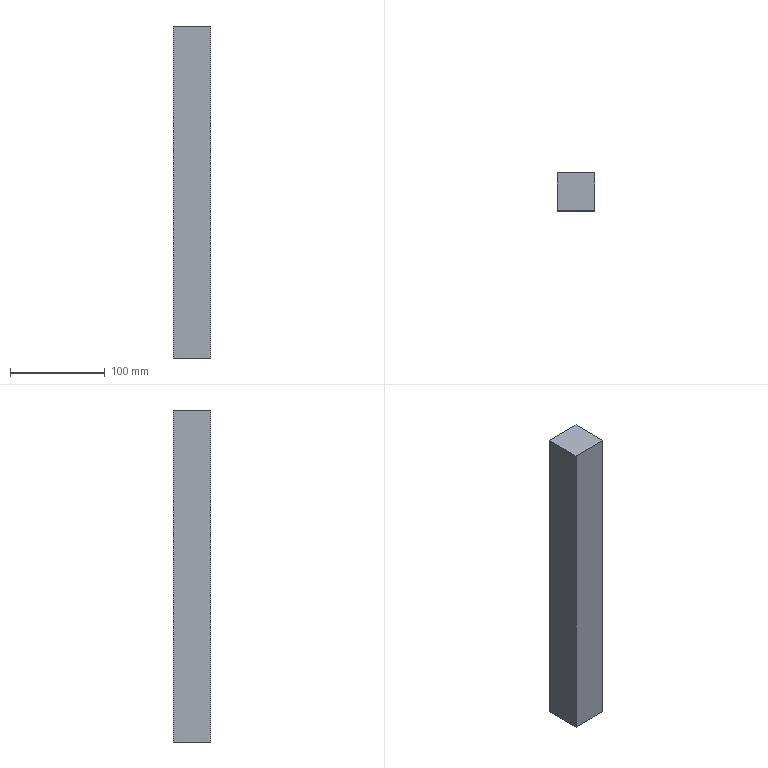Part | STEP file | Profile | 1 solid | 6 faces | box 40 x 40 x 350 mm | volume 560000 mm3 | plane 6
STEP:
#1=CARTESIAN_POINT('',(0.,0.,0.));
#2=DIRECTION('',(0.,0.,1.));
#3=DIRECTION('',(1.,0.,0.));
#4=AXIS2_PLACEMENT_3D('',#1,#2,#3);
#5=CARTESIAN_POINT('',(20.,-20.,350.));
#6=VERTEX_POINT('',#5);
#7=CARTESIAN_POINT('',(20.,-20.,0.));
#8=VERTEX_POINT('',#7);
#9=CARTESIAN_POINT('',(20.,-20.,350.));
#10=DIRECTION('',(0.,0.,-1.));
#11=VECTOR('',#10,1.);
#12=LINE('',#9,#11);
#13=CARTESIAN_POINT('',(-20.,-20.,350.));
#14=DIRECTION('',(0.,1.,0.));
#15=DIRECTION('',(0.,0.,1.));
#16=AXIS2_PLACEMENT_3D('',#13,#14,#15);
#17=PLANE('',#16);
#18=CARTESIAN_POINT('',(0.,40.));
#19=DIRECTION('',(-1.,0.));
#20=VECTOR('',#19,1.);
#21=LINE('',#18,#20);
#22=(GEOMETRIC_REPRESENTATION_CONTEXT(2)PARAMETRIC_REPRESENTATION_CONTEXT()REPRESENTATION_CONTEXT('',''));
#23=DEFINITIONAL_REPRESENTATION('',(#21),#22);
#24=PCURVE('',#17,#23);
#25=CARTESIAN_POINT('',(20.,20.,350.));
#26=DIRECTION('',(-1.,0.,0.));
#27=DIRECTION('',(0.,-1.,0.));
#28=AXIS2_PLACEMENT_3D('',#25,#26,#27);
#29=PLANE('',#28);
#30=CARTESIAN_POINT('',(40.,0.));
#31=DIRECTION('',(0.,-1.));
#32=VECTOR('',#31,1.);
#33=LINE('',#30,#32);
#34=(GEOMETRIC_REPRESENTATION_CONTEXT(2)PARAMETRIC_REPRESENTATION_CONTEXT()REPRESENTATION_CONTEXT('',''));
#35=DEFINITIONAL_REPRESENTATION('',(#33),#34);
#36=PCURVE('',#29,#35);
#37=SURFACE_CURVE('',#12,(#24,#36),.PCURVE_S1.);
#38=EDGE_CURVE('',#6,#8,#37,.T.);
#39=ORIENTED_EDGE('',*,*,#38,.F.);
#40=CARTESIAN_POINT('',(-20.,-20.,350.));
#41=VERTEX_POINT('',#40);
#42=CARTESIAN_POINT('',(-20.,-20.,350.));
#43=DIRECTION('',(1.,0.,0.));
#44=VECTOR('',#43,1.);
#45=LINE('',#42,#44);
#46=CARTESIAN_POINT('',(0.,0.));
#47=DIRECTION('',(0.,1.));
#48=VECTOR('',#47,1.);
#49=LINE('',#46,#48);
#50=(GEOMETRIC_REPRESENTATION_CONTEXT(2)PARAMETRIC_REPRESENTATION_CONTEXT()REPRESENTATION_CONTEXT('',''));
#51=DEFINITIONAL_REPRESENTATION('',(#49),#50);
#52=PCURVE('',#17,#51);
#53=CARTESIAN_POINT('',(0.,0.,350.));
#54=DIRECTION('',(0.,0.,1.));
#55=DIRECTION('',(1.,0.,0.));
#56=AXIS2_PLACEMENT_3D('',#53,#54,#55);
#57=PLANE('',#56);
#58=CARTESIAN_POINT('',(-20.,-20.));
#59=DIRECTION('',(1.,0.));
#60=VECTOR('',#59,1.);
#61=LINE('',#58,#60);
#62=(GEOMETRIC_REPRESENTATION_CONTEXT(2)PARAMETRIC_REPRESENTATION_CONTEXT()REPRESENTATION_CONTEXT('',''));
#63=DEFINITIONAL_REPRESENTATION('',(#61),#62);
#64=PCURVE('',#57,#63);
#65=SURFACE_CURVE('',#45,(#52,#64),.PCURVE_S1.);
#66=EDGE_CURVE('',#41,#6,#65,.T.);
#67=ORIENTED_EDGE('',*,*,#66,.F.);
#68=CARTESIAN_POINT('',(-20.,-20.,0.));
#69=VERTEX_POINT('',#68);
#70=CARTESIAN_POINT('',(-20.,-20.,350.));
#71=DIRECTION('',(0.,0.,1.));
#72=VECTOR('',#71,1.);
#73=LINE('',#70,#72);
#74=CARTESIAN_POINT('',(0.,0.));
#75=DIRECTION('',(1.,0.));
#76=VECTOR('',#75,1.);
#77=LINE('',#74,#76);
#78=(GEOMETRIC_REPRESENTATION_CONTEXT(2)PARAMETRIC_REPRESENTATION_CONTEXT()REPRESENTATION_CONTEXT('',''));
#79=DEFINITIONAL_REPRESENTATION('',(#77),#78);
#80=PCURVE('',#17,#79);
#81=CARTESIAN_POINT('',(-20.,20.,350.));
#82=DIRECTION('',(1.,0.,0.));
#83=DIRECTION('',(0.,1.,0.));
#84=AXIS2_PLACEMENT_3D('',#81,#82,#83);
#85=PLANE('',#84);
#86=CARTESIAN_POINT('',(-40.,0.));
#87=DIRECTION('',(0.,1.));
#88=VECTOR('',#87,1.);
#89=LINE('',#86,#88);
#90=(GEOMETRIC_REPRESENTATION_CONTEXT(2)PARAMETRIC_REPRESENTATION_CONTEXT()REPRESENTATION_CONTEXT('',''));
#91=DEFINITIONAL_REPRESENTATION('',(#89),#90);
#92=PCURVE('',#85,#91);
#93=SURFACE_CURVE('',#73,(#80,#92),.PCURVE_S1.);
#94=EDGE_CURVE('',#69,#41,#93,.T.);
#95=ORIENTED_EDGE('',*,*,#94,.F.);
#96=CARTESIAN_POINT('',(-20.,-20.,0.));
#97=DIRECTION('',(-1.,0.,0.));
#98=VECTOR('',#97,1.);
#99=LINE('',#96,#98);
#100=CARTESIAN_POINT('',(-350.,0.));
#101=DIRECTION('',(0.,-1.));
#102=VECTOR('',#101,1.);
#103=LINE('',#100,#102);
#104=(GEOMETRIC_REPRESENTATION_CONTEXT(2)PARAMETRIC_REPRESENTATION_CONTEXT()REPRESENTATION_CONTEXT('',''));
#105=DEFINITIONAL_REPRESENTATION('',(#103),#104);
#106=PCURVE('',#17,#105);
#107=CARTESIAN_POINT('',(0.,0.,0.));
#108=DIRECTION('',(0.,0.,1.));
#109=DIRECTION('',(1.,0.,0.));
#110=AXIS2_PLACEMENT_3D('',#107,#108,#109);
#111=PLANE('',#110);
#112=CARTESIAN_POINT('',(-20.,-20.));
#113=DIRECTION('',(-1.,0.));
#114=VECTOR('',#113,1.);
#115=LINE('',#112,#114);
#116=(GEOMETRIC_REPRESENTATION_CONTEXT(2)PARAMETRIC_REPRESENTATION_CONTEXT()REPRESENTATION_CONTEXT('',''));
#117=DEFINITIONAL_REPRESENTATION('',(#115),#116);
#118=PCURVE('',#111,#117);
#119=SURFACE_CURVE('',#99,(#106,#118),.PCURVE_S1.);
#120=EDGE_CURVE('',#8,#69,#119,.T.);
#121=ORIENTED_EDGE('',*,*,#120,.F.);
#122=EDGE_LOOP('',(#39,#67,#95,#121));
#123=FACE_BOUND('',#122,.T.);
#124=ADVANCED_FACE('',(#123),#17,.F.);
#125=ORIENTED_EDGE('',*,*,#120,.T.);
#126=CARTESIAN_POINT('',(-20.,20.,0.));
#127=VERTEX_POINT('',#126);
#128=CARTESIAN_POINT('',(-20.,0.,0.));
#129=DIRECTION('',(0.,-1.,0.));
#130=VECTOR('',#129,1.);
#131=LINE('',#128,#130);
#132=CARTESIAN_POINT('',(-20.,0.));
#133=DIRECTION('',(0.,-1.));
#134=VECTOR('',#133,1.);
#135=LINE('',#132,#134);
#136=(GEOMETRIC_REPRESENTATION_CONTEXT(2)PARAMETRIC_REPRESENTATION_CONTEXT()REPRESENTATION_CONTEXT('',''));
#137=DEFINITIONAL_REPRESENTATION('',(#135),#136);
#138=PCURVE('',#111,#137);
#139=CARTESIAN_POINT('',(-20.,-350.));
#140=DIRECTION('',(-1.,0.));
#141=VECTOR('',#140,1.);
#142=LINE('',#139,#141);
#143=(GEOMETRIC_REPRESENTATION_CONTEXT(2)PARAMETRIC_REPRESENTATION_CONTEXT()REPRESENTATION_CONTEXT('',''));
#144=DEFINITIONAL_REPRESENTATION('',(#142),#143);
#145=PCURVE('',#85,#144);
#146=SURFACE_CURVE('',#131,(#138,#145),.PCURVE_S1.);
#147=EDGE_CURVE('',#127,#69,#146,.T.);
#148=ORIENTED_EDGE('',*,*,#147,.F.);
#149=CARTESIAN_POINT('',(20.,20.,0.));
#150=VERTEX_POINT('',#149);
#151=CARTESIAN_POINT('',(0.,20.,0.));
#152=DIRECTION('',(-1.,0.,0.));
#153=VECTOR('',#152,1.);
#154=LINE('',#151,#153);
#155=CARTESIAN_POINT('',(0.,20.));
#156=DIRECTION('',(-1.,0.));
#157=VECTOR('',#156,1.);
#158=LINE('',#155,#157);
#159=(GEOMETRIC_REPRESENTATION_CONTEXT(2)PARAMETRIC_REPRESENTATION_CONTEXT()REPRESENTATION_CONTEXT('',''));
#160=DEFINITIONAL_REPRESENTATION('',(#158),#159);
#161=PCURVE('',#111,#160);
#162=CARTESIAN_POINT('',(-20.,20.,350.));
#163=DIRECTION('',(0.,-1.,0.));
#164=DIRECTION('',(0.,0.,-1.));
#165=AXIS2_PLACEMENT_3D('',#162,#163,#164);
#166=PLANE('',#165);
#167=CARTESIAN_POINT('',(350.,20.));
#168=DIRECTION('',(0.,-1.));
#169=VECTOR('',#168,1.);
#170=LINE('',#167,#169);
#171=(GEOMETRIC_REPRESENTATION_CONTEXT(2)PARAMETRIC_REPRESENTATION_CONTEXT()REPRESENTATION_CONTEXT('',''));
#172=DEFINITIONAL_REPRESENTATION('',(#170),#171);
#173=PCURVE('',#166,#172);
#174=SURFACE_CURVE('',#154,(#161,#173),.PCURVE_S1.);
#175=EDGE_CURVE('',#150,#127,#174,.T.);
#176=ORIENTED_EDGE('',*,*,#175,.F.);
#177=CARTESIAN_POINT('',(20.,0.,0.));
#178=DIRECTION('',(0.,1.,0.));
#179=VECTOR('',#178,1.);
#180=LINE('',#177,#179);
#181=CARTESIAN_POINT('',(20.,0.));
#182=DIRECTION('',(0.,1.));
#183=VECTOR('',#182,1.);
#184=LINE('',#181,#183);
#185=(GEOMETRIC_REPRESENTATION_CONTEXT(2)PARAMETRIC_REPRESENTATION_CONTEXT()REPRESENTATION_CONTEXT('',''));
#186=DEFINITIONAL_REPRESENTATION('',(#184),#185);
#187=PCURVE('',#111,#186);
#188=CARTESIAN_POINT('',(20.,-350.));
#189=DIRECTION('',(-1.,0.));
#190=VECTOR('',#189,1.);
#191=LINE('',#188,#190);
#192=(GEOMETRIC_REPRESENTATION_CONTEXT(2)PARAMETRIC_REPRESENTATION_CONTEXT()REPRESENTATION_CONTEXT('',''));
#193=DEFINITIONAL_REPRESENTATION('',(#191),#192);
#194=PCURVE('',#29,#193);
#195=SURFACE_CURVE('',#180,(#187,#194),.PCURVE_S1.);
#196=EDGE_CURVE('',#8,#150,#195,.T.);
#197=ORIENTED_EDGE('',*,*,#196,.F.);
#198=EDGE_LOOP('',(#125,#148,#176,#197));
#199=FACE_BOUND('',#198,.T.);
#200=ADVANCED_FACE('',(#199),#111,.F.);
#201=CARTESIAN_POINT('',(20.,20.,350.));
#202=VERTEX_POINT('',#201);
#203=CARTESIAN_POINT('',(20.,20.,350.));
#204=DIRECTION('',(0.,0.,-1.));
#205=VECTOR('',#204,1.);
#206=LINE('',#203,#205);
#207=CARTESIAN_POINT('',(0.,0.));
#208=DIRECTION('',(0.,-1.));
#209=VECTOR('',#208,1.);
#210=LINE('',#207,#209);
#211=(GEOMETRIC_REPRESENTATION_CONTEXT(2)PARAMETRIC_REPRESENTATION_CONTEXT()REPRESENTATION_CONTEXT('',''));
#212=DEFINITIONAL_REPRESENTATION('',(#210),#211);
#213=PCURVE('',#29,#212);
#214=CARTESIAN_POINT('',(0.,40.));
#215=DIRECTION('',(1.,0.));
#216=VECTOR('',#215,1.);
#217=LINE('',#214,#216);
#218=(GEOMETRIC_REPRESENTATION_CONTEXT(2)PARAMETRIC_REPRESENTATION_CONTEXT()REPRESENTATION_CONTEXT('',''));
#219=DEFINITIONAL_REPRESENTATION('',(#217),#218);
#220=PCURVE('',#166,#219);
#221=SURFACE_CURVE('',#206,(#213,#220),.PCURVE_S1.);
#222=EDGE_CURVE('',#202,#150,#221,.T.);
#223=ORIENTED_EDGE('',*,*,#222,.F.);
#224=CARTESIAN_POINT('',(20.,20.,350.));
#225=DIRECTION('',(0.,1.,0.));
#226=VECTOR('',#225,1.);
#227=LINE('',#224,#226);
#228=CARTESIAN_POINT('',(0.,0.));
#229=DIRECTION('',(-1.,0.));
#230=VECTOR('',#229,1.);
#231=LINE('',#228,#230);
#232=(GEOMETRIC_REPRESENTATION_CONTEXT(2)PARAMETRIC_REPRESENTATION_CONTEXT()REPRESENTATION_CONTEXT('',''));
#233=DEFINITIONAL_REPRESENTATION('',(#231),#232);
#234=PCURVE('',#29,#233);
#235=CARTESIAN_POINT('',(20.,20.));
#236=DIRECTION('',(0.,1.));
#237=VECTOR('',#236,1.);
#238=LINE('',#235,#237);
#239=(GEOMETRIC_REPRESENTATION_CONTEXT(2)PARAMETRIC_REPRESENTATION_CONTEXT()REPRESENTATION_CONTEXT('',''));
#240=DEFINITIONAL_REPRESENTATION('',(#238),#239);
#241=PCURVE('',#57,#240);
#242=SURFACE_CURVE('',#227,(#234,#241),.PCURVE_S1.);
#243=EDGE_CURVE('',#6,#202,#242,.T.);
#244=ORIENTED_EDGE('',*,*,#243,.F.);
#245=ORIENTED_EDGE('',*,*,#38,.T.);
#246=ORIENTED_EDGE('',*,*,#196,.T.);
#247=EDGE_LOOP('',(#223,#244,#245,#246));
#248=FACE_BOUND('',#247,.T.);
#249=ADVANCED_FACE('',(#248),#29,.F.);
#250=CARTESIAN_POINT('',(-20.,20.,350.));
#251=VERTEX_POINT('',#250);
#252=CARTESIAN_POINT('',(-20.,0.,350.));
#253=DIRECTION('',(0.,-1.,0.));
#254=VECTOR('',#253,1.);
#255=LINE('',#252,#254);
#256=CARTESIAN_POINT('',(-20.,0.));
#257=DIRECTION('',(0.,-1.));
#258=VECTOR('',#257,1.);
#259=LINE('',#256,#258);
#260=(GEOMETRIC_REPRESENTATION_CONTEXT(2)PARAMETRIC_REPRESENTATION_CONTEXT()REPRESENTATION_CONTEXT('',''));
#261=DEFINITIONAL_REPRESENTATION('',(#259),#260);
#262=PCURVE('',#57,#261);
#263=CARTESIAN_POINT('',(-20.,0.));
#264=DIRECTION('',(-1.,0.));
#265=VECTOR('',#264,1.);
#266=LINE('',#263,#265);
#267=(GEOMETRIC_REPRESENTATION_CONTEXT(2)PARAMETRIC_REPRESENTATION_CONTEXT()REPRESENTATION_CONTEXT('',''));
#268=DEFINITIONAL_REPRESENTATION('',(#266),#267);
#269=PCURVE('',#85,#268);
#270=SURFACE_CURVE('',#255,(#262,#269),.PCURVE_S1.);
#271=EDGE_CURVE('',#251,#41,#270,.T.);
#272=ORIENTED_EDGE('',*,*,#271,.T.);
#273=ORIENTED_EDGE('',*,*,#66,.T.);
#274=ORIENTED_EDGE('',*,*,#243,.T.);
#275=CARTESIAN_POINT('',(0.,20.,350.));
#276=DIRECTION('',(-1.,0.,0.));
#277=VECTOR('',#276,1.);
#278=LINE('',#275,#277);
#279=CARTESIAN_POINT('',(0.,20.));
#280=DIRECTION('',(-1.,0.));
#281=VECTOR('',#280,1.);
#282=LINE('',#279,#281);
#283=(GEOMETRIC_REPRESENTATION_CONTEXT(2)PARAMETRIC_REPRESENTATION_CONTEXT()REPRESENTATION_CONTEXT('',''));
#284=DEFINITIONAL_REPRESENTATION('',(#282),#283);
#285=PCURVE('',#57,#284);
#286=CARTESIAN_POINT('',(0.,20.));
#287=DIRECTION('',(0.,-1.));
#288=VECTOR('',#287,1.);
#289=LINE('',#286,#288);
#290=(GEOMETRIC_REPRESENTATION_CONTEXT(2)PARAMETRIC_REPRESENTATION_CONTEXT()REPRESENTATION_CONTEXT('',''));
#291=DEFINITIONAL_REPRESENTATION('',(#289),#290);
#292=PCURVE('',#166,#291);
#293=SURFACE_CURVE('',#278,(#285,#292),.PCURVE_S1.);
#294=EDGE_CURVE('',#202,#251,#293,.T.);
#295=ORIENTED_EDGE('',*,*,#294,.T.);
#296=EDGE_LOOP('',(#272,#273,#274,#295));
#297=FACE_BOUND('',#296,.T.);
#298=ADVANCED_FACE('',(#297),#57,.T.);
#299=ORIENTED_EDGE('',*,*,#94,.T.);
#300=ORIENTED_EDGE('',*,*,#271,.F.);
#301=CARTESIAN_POINT('',(-20.,20.,350.));
#302=DIRECTION('',(0.,0.,1.));
#303=VECTOR('',#302,1.);
#304=LINE('',#301,#303);
#305=CARTESIAN_POINT('',(0.,0.));
#306=DIRECTION('',(0.,1.));
#307=VECTOR('',#306,1.);
#308=LINE('',#305,#307);
#309=(GEOMETRIC_REPRESENTATION_CONTEXT(2)PARAMETRIC_REPRESENTATION_CONTEXT()REPRESENTATION_CONTEXT('',''));
#310=DEFINITIONAL_REPRESENTATION('',(#308),#309);
#311=PCURVE('',#85,#310);
#312=CARTESIAN_POINT('',(0.,0.));
#313=DIRECTION('',(-1.,0.));
#314=VECTOR('',#313,1.);
#315=LINE('',#312,#314);
#316=(GEOMETRIC_REPRESENTATION_CONTEXT(2)PARAMETRIC_REPRESENTATION_CONTEXT()REPRESENTATION_CONTEXT('',''));
#317=DEFINITIONAL_REPRESENTATION('',(#315),#316);
#318=PCURVE('',#166,#317);
#319=SURFACE_CURVE('',#304,(#311,#318),.PCURVE_S1.);
#320=EDGE_CURVE('',#127,#251,#319,.T.);
#321=ORIENTED_EDGE('',*,*,#320,.F.);
#322=ORIENTED_EDGE('',*,*,#147,.T.);
#323=EDGE_LOOP('',(#299,#300,#321,#322));
#324=FACE_BOUND('',#323,.T.);
#325=ADVANCED_FACE('',(#324),#85,.F.);
#326=ORIENTED_EDGE('',*,*,#320,.T.);
#327=ORIENTED_EDGE('',*,*,#294,.F.);
#328=ORIENTED_EDGE('',*,*,#222,.T.);
#329=ORIENTED_EDGE('',*,*,#175,.T.);
#330=EDGE_LOOP('',(#326,#327,#328,#329));
#331=FACE_BOUND('',#330,.T.);
#332=ADVANCED_FACE('',(#331),#166,.F.);
#333=CLOSED_SHELL('',(#124,#200,#249,#298,#325,#332));
#334=MANIFOLD_SOLID_BREP('',#333);
#335=(LENGTH_UNIT()NAMED_UNIT(*)SI_UNIT(.MILLI.,.METRE.));
#336=UNCERTAINTY_MEASURE_WITH_UNIT(LENGTH_MEASURE(0.0000001),#335,'','');
#337=(NAMED_UNIT(*)PLANE_ANGLE_UNIT()SI_UNIT($,.RADIAN.));
#338=(NAMED_UNIT(*)SI_UNIT($,.STERADIAN.)SOLID_ANGLE_UNIT());
#339=(GEOMETRIC_REPRESENTATION_CONTEXT(3)GLOBAL_UNCERTAINTY_ASSIGNED_CONTEXT((#336))GLOBAL_UNIT_ASSIGNED_CONTEXT((#335,#337,#338))REPRESENTATION_CONTEXT('',''));
#340=ADVANCED_BREP_SHAPE_REPRESENTATION('',(#4,#334),#339);